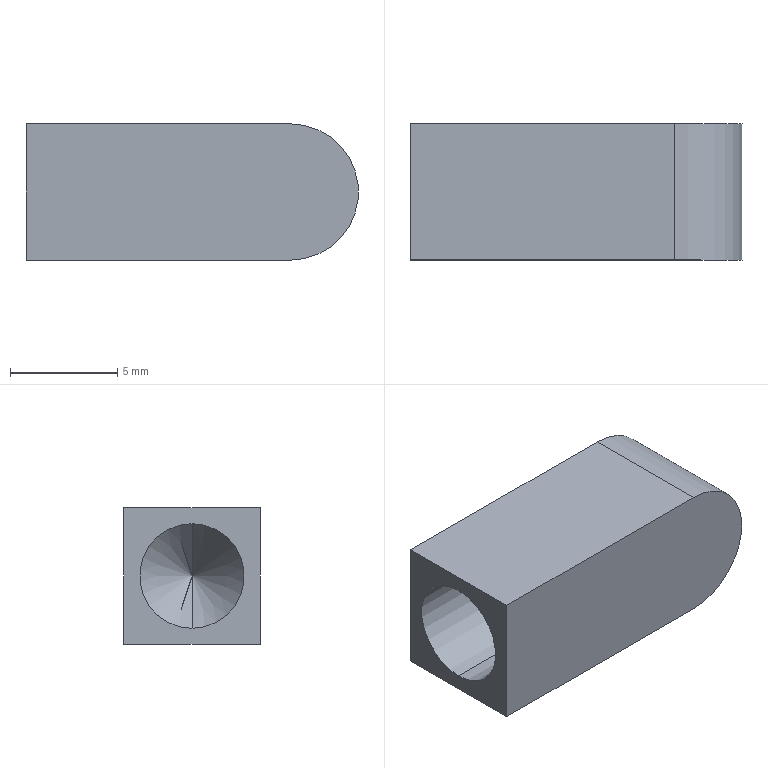Part | SolidWorks | features Extrusion 1, ICE 1, RevCut 1 | 1 solid | 10 faces | box 15.494 x 6.35 x 6.35 mm | volume 372.244 mm3 | plane 5 | cylinder 3 | cone 2 | commonest cylinder face diameters 4.877 x2 6.35 x1
STEP:
#1=CARTESIAN_POINT('',(0.5479,0.,0.));
#2=VERTEX_POINT('',#1);
#3=CARTESIAN_POINT('',(0.4375,0.,0.096));
#4=VERTEX_POINT('',#3);
#5=CARTESIAN_POINT('',(0.4375,0.,0.096));
#6=DIRECTION('',(-0.7547,0.,0.6561));
#7=VECTOR('',#6,39.37);
#8=LINE('',#5,#7);
#9=EDGE_CURVE('',#2,#4,#8,.T.);
#10=ORIENTED_EDGE('',*,*,#9,.F.);
#11=CARTESIAN_POINT('',(0.4375,0.,-0.096));
#12=VERTEX_POINT('',#11);
#13=CARTESIAN_POINT('',(0.4375,0.,-0.096));
#14=DIRECTION('',(-0.7547,0.,-0.6561));
#15=VECTOR('',#14,39.37);
#16=LINE('',#13,#15);
#17=EDGE_CURVE('',#2,#12,#16,.T.);
#18=ORIENTED_EDGE('',*,*,#17,.T.);
#19=CARTESIAN_POINT('',(0.4375,0.,0.));
#20=DIRECTION('',(-1.,0.,0.));
#21=DIRECTION('',(0.,0.,1.));
#22=AXIS2_PLACEMENT_3D('',#19,#20,#21);
#23=CIRCLE('',#22,0.096);
#24=EDGE_CURVE('',#12,#4,#23,.T.);
#25=ORIENTED_EDGE('',*,*,#24,.T.);
#26=EDGE_LOOP('',(#10,#18,#25));
#27=FACE_OUTER_BOUND('',#26,.T.);
#28=CARTESIAN_POINT('',(0.4375,0.,0.));
#29=DIRECTION('',(-1.,0.,0.));
#30=DIRECTION('',(0.,0.,1.));
#31=AXIS2_PLACEMENT_3D('',#28,#29,#30);
#32=CONICAL_SURFACE('',#31,0.096,0.7156);
#33=ADVANCED_FACE('',(#27),#32,.F.);
#34=ORIENTED_EDGE('',*,*,#24,.F.);
#35=CARTESIAN_POINT('',(0.,0.,-0.096));
#36=VERTEX_POINT('',#35);
#37=CARTESIAN_POINT('',(0.4375,0.,-0.096));
#38=DIRECTION('',(-1.,0.,0.));
#39=VECTOR('',#38,39.37);
#40=LINE('',#37,#39);
#41=EDGE_CURVE('',#12,#36,#40,.T.);
#42=ORIENTED_EDGE('',*,*,#41,.T.);
#43=CARTESIAN_POINT('',(0.,0.,0.096));
#44=VERTEX_POINT('',#43);
#45=CARTESIAN_POINT('',(0.,0.,0.));
#46=DIRECTION('',(-1.,0.,0.));
#47=DIRECTION('',(0.,0.,1.));
#48=AXIS2_PLACEMENT_3D('',#45,#46,#47);
#49=CIRCLE('',#48,0.096);
#50=EDGE_CURVE('',#36,#44,#49,.T.);
#51=ORIENTED_EDGE('',*,*,#50,.T.);
#52=CARTESIAN_POINT('',(0.4375,0.,0.096));
#53=DIRECTION('',(-1.,0.,0.));
#54=VECTOR('',#53,39.37);
#55=LINE('',#52,#54);
#56=EDGE_CURVE('',#4,#44,#55,.T.);
#57=ORIENTED_EDGE('',*,*,#56,.F.);
#58=EDGE_LOOP('',(#34,#42,#51,#57));
#59=FACE_OUTER_BOUND('',#58,.T.);
#60=CARTESIAN_POINT('',(0.4375,0.,0.));
#61=DIRECTION('',(-1.,0.,0.));
#62=DIRECTION('',(0.,0.,1.));
#63=AXIS2_PLACEMENT_3D('',#60,#61,#62);
#64=CYLINDRICAL_SURFACE('',#63,0.096);
#65=ADVANCED_FACE('',(#59),#64,.F.);
#66=CARTESIAN_POINT('',(0.,0.,0.));
#67=DIRECTION('',(-1.,0.,0.));
#68=DIRECTION('',(0.,0.,1.));
#69=AXIS2_PLACEMENT_3D('',#66,#67,#68);
#70=CIRCLE('',#69,0.096);
#71=EDGE_CURVE('',#44,#36,#70,.T.);
#72=ORIENTED_EDGE('',*,*,#71,.F.);
#73=ORIENTED_EDGE('',*,*,#50,.F.);
#74=EDGE_LOOP('',(#72,#73));
#75=FACE_BOUND('',#74,.T.);
#76=CARTESIAN_POINT('',(0.,-0.125,-0.125));
#77=VERTEX_POINT('',#76);
#78=CARTESIAN_POINT('',(0.,-0.125,0.125));
#79=VERTEX_POINT('',#78);
#80=CARTESIAN_POINT('',(0.,-0.125,-0.125));
#81=DIRECTION('',(0.,0.,1.));
#82=VECTOR('',#81,39.37);
#83=LINE('',#80,#82);
#84=EDGE_CURVE('',#77,#79,#83,.T.);
#85=ORIENTED_EDGE('',*,*,#84,.T.);
#86=CARTESIAN_POINT('',(0.,0.125,0.125));
#87=VERTEX_POINT('',#86);
#88=CARTESIAN_POINT('',(0.,0.125,0.125));
#89=DIRECTION('',(0.,-1.,0.));
#90=VECTOR('',#89,39.37);
#91=LINE('',#88,#90);
#92=EDGE_CURVE('',#87,#79,#91,.T.);
#93=ORIENTED_EDGE('',*,*,#92,.F.);
#94=CARTESIAN_POINT('',(0.,0.125,-0.125));
#95=VERTEX_POINT('',#94);
#96=CARTESIAN_POINT('',(0.,0.125,-0.125));
#97=DIRECTION('',(0.,0.,1.));
#98=VECTOR('',#97,39.37);
#99=LINE('',#96,#98);
#100=EDGE_CURVE('',#95,#87,#99,.T.);
#101=ORIENTED_EDGE('',*,*,#100,.F.);
#102=CARTESIAN_POINT('',(0.,0.125,-0.125));
#103=DIRECTION('',(0.,-1.,0.));
#104=VECTOR('',#103,39.37);
#105=LINE('',#102,#104);
#106=EDGE_CURVE('',#95,#77,#105,.T.);
#107=ORIENTED_EDGE('',*,*,#106,.T.);
#108=EDGE_LOOP('',(#85,#93,#101,#107));
#109=FACE_OUTER_BOUND('',#108,.T.);
#110=CARTESIAN_POINT('',(0.,0.125,-0.125));
#111=DIRECTION('',(1.,0.,0.));
#112=DIRECTION('',(0.,0.,-1.));
#113=AXIS2_PLACEMENT_3D('',#110,#111,#112);
#114=PLANE('',#113);
#115=ADVANCED_FACE('',(#75,#109),#114,.F.);
#116=CARTESIAN_POINT('',(0.485,-0.125,0.125));
#117=VERTEX_POINT('',#116);
#118=CARTESIAN_POINT('',(0.,-0.125,0.125));
#119=DIRECTION('',(1.,0.,0.));
#120=VECTOR('',#119,39.37);
#121=LINE('',#118,#120);
#122=EDGE_CURVE('',#79,#117,#121,.T.);
#123=ORIENTED_EDGE('',*,*,#122,.T.);
#124=CARTESIAN_POINT('',(0.485,0.125,0.125));
#125=VERTEX_POINT('',#124);
#126=CARTESIAN_POINT('',(0.485,0.125,0.125));
#127=DIRECTION('',(0.,-1.,0.));
#128=VECTOR('',#127,39.37);
#129=LINE('',#126,#128);
#130=EDGE_CURVE('',#125,#117,#129,.T.);
#131=ORIENTED_EDGE('',*,*,#130,.F.);
#132=CARTESIAN_POINT('',(0.,0.125,0.125));
#133=DIRECTION('',(1.,0.,0.));
#134=VECTOR('',#133,39.37);
#135=LINE('',#132,#134);
#136=EDGE_CURVE('',#87,#125,#135,.T.);
#137=ORIENTED_EDGE('',*,*,#136,.F.);
#138=ORIENTED_EDGE('',*,*,#92,.T.);
#139=EDGE_LOOP('',(#123,#131,#137,#138));
#140=FACE_OUTER_BOUND('',#139,.T.);
#141=CARTESIAN_POINT('',(0.,0.125,0.125));
#142=DIRECTION('',(0.,0.,-1.));
#143=DIRECTION('',(-1.,0.,0.));
#144=AXIS2_PLACEMENT_3D('',#141,#142,#143);
#145=PLANE('',#144);
#146=ADVANCED_FACE('',(#140),#145,.F.);
#147=CARTESIAN_POINT('',(0.485,-0.125,-0.125));
#148=VERTEX_POINT('',#147);
#149=CARTESIAN_POINT('',(0.485,-0.125,0.));
#150=DIRECTION('',(0.,1.,0.));
#151=DIRECTION('',(0.,0.,1.));
#152=AXIS2_PLACEMENT_3D('',#149,#150,#151);
#153=CIRCLE('',#152,0.125);
#154=EDGE_CURVE('',#117,#148,#153,.T.);
#155=ORIENTED_EDGE('',*,*,#154,.T.);
#156=CARTESIAN_POINT('',(0.485,0.125,-0.125));
#157=VERTEX_POINT('',#156);
#158=CARTESIAN_POINT('',(0.485,0.125,-0.125));
#159=DIRECTION('',(0.,-1.,0.));
#160=VECTOR('',#159,39.37);
#161=LINE('',#158,#160);
#162=EDGE_CURVE('',#157,#148,#161,.T.);
#163=ORIENTED_EDGE('',*,*,#162,.F.);
#164=CARTESIAN_POINT('',(0.485,0.125,0.));
#165=DIRECTION('',(0.,1.,0.));
#166=DIRECTION('',(0.,0.,1.));
#167=AXIS2_PLACEMENT_3D('',#164,#165,#166);
#168=CIRCLE('',#167,0.125);
#169=EDGE_CURVE('',#125,#157,#168,.T.);
#170=ORIENTED_EDGE('',*,*,#169,.F.);
#171=ORIENTED_EDGE('',*,*,#130,.T.);
#172=EDGE_LOOP('',(#155,#163,#170,#171));
#173=FACE_OUTER_BOUND('',#172,.T.);
#174=CARTESIAN_POINT('',(0.485,0.125,0.));
#175=DIRECTION('',(0.,-1.,0.));
#176=DIRECTION('',(0.,0.,-1.));
#177=AXIS2_PLACEMENT_3D('',#174,#175,#176);
#178=CYLINDRICAL_SURFACE('',#177,0.125);
#179=ADVANCED_FACE('',(#173),#178,.T.);
#180=CARTESIAN_POINT('',(0.,-0.125,-0.125));
#181=DIRECTION('',(-1.,0.,0.));
#182=VECTOR('',#181,39.37);
#183=LINE('',#180,#182);
#184=EDGE_CURVE('',#148,#77,#183,.T.);
#185=ORIENTED_EDGE('',*,*,#184,.T.);
#186=ORIENTED_EDGE('',*,*,#106,.F.);
#187=CARTESIAN_POINT('',(0.,0.125,-0.125));
#188=DIRECTION('',(-1.,0.,0.));
#189=VECTOR('',#188,39.37);
#190=LINE('',#187,#189);
#191=EDGE_CURVE('',#157,#95,#190,.T.);
#192=ORIENTED_EDGE('',*,*,#191,.F.);
#193=ORIENTED_EDGE('',*,*,#162,.T.);
#194=EDGE_LOOP('',(#185,#186,#192,#193));
#195=FACE_OUTER_BOUND('',#194,.T.);
#196=CARTESIAN_POINT('',(0.,0.125,-0.125));
#197=DIRECTION('',(0.,0.,1.));
#198=DIRECTION('',(1.,0.,0.));
#199=AXIS2_PLACEMENT_3D('',#196,#197,#198);
#200=PLANE('',#199);
#201=ADVANCED_FACE('',(#195),#200,.F.);
#202=ORIENTED_EDGE('',*,*,#100,.T.);
#203=ORIENTED_EDGE('',*,*,#136,.T.);
#204=ORIENTED_EDGE('',*,*,#169,.T.);
#205=ORIENTED_EDGE('',*,*,#191,.T.);
#206=EDGE_LOOP('',(#202,#203,#204,#205));
#207=FACE_OUTER_BOUND('',#206,.T.);
#208=CARTESIAN_POINT('',(0.485,0.125,0.));
#209=DIRECTION('',(0.,1.,0.));
#210=DIRECTION('',(0.,0.,1.));
#211=AXIS2_PLACEMENT_3D('',#208,#209,#210);
#212=PLANE('',#211);
#213=ADVANCED_FACE('',(#207),#212,.T.);
#214=ORIENTED_EDGE('',*,*,#84,.F.);
#215=ORIENTED_EDGE('',*,*,#184,.F.);
#216=ORIENTED_EDGE('',*,*,#154,.F.);
#217=ORIENTED_EDGE('',*,*,#122,.F.);
#218=EDGE_LOOP('',(#214,#215,#216,#217));
#219=FACE_OUTER_BOUND('',#218,.T.);
#220=CARTESIAN_POINT('',(0.485,-0.125,0.));
#221=DIRECTION('',(0.,1.,0.));
#222=DIRECTION('',(0.,0.,1.));
#223=AXIS2_PLACEMENT_3D('',#220,#221,#222);
#224=PLANE('',#223);
#225=ADVANCED_FACE('',(#219),#224,.F.);
#226=ORIENTED_EDGE('',*,*,#41,.F.);
#227=CARTESIAN_POINT('',(0.4375,0.,0.));
#228=DIRECTION('',(-1.,0.,0.));
#229=DIRECTION('',(0.,0.,1.));
#230=AXIS2_PLACEMENT_3D('',#227,#228,#229);
#231=CIRCLE('',#230,0.096);
#232=EDGE_CURVE('',#4,#12,#231,.T.);
#233=ORIENTED_EDGE('',*,*,#232,.F.);
#234=ORIENTED_EDGE('',*,*,#56,.T.);
#235=ORIENTED_EDGE('',*,*,#71,.T.);
#236=EDGE_LOOP('',(#226,#233,#234,#235));
#237=FACE_OUTER_BOUND('',#236,.T.);
#238=CARTESIAN_POINT('',(0.4375,0.,0.));
#239=DIRECTION('',(-1.,0.,0.));
#240=DIRECTION('',(0.,0.,1.));
#241=AXIS2_PLACEMENT_3D('',#238,#239,#240);
#242=CYLINDRICAL_SURFACE('',#241,0.096);
#243=ADVANCED_FACE('',(#237),#242,.F.);
#244=ORIENTED_EDGE('',*,*,#17,.F.);
#245=ORIENTED_EDGE('',*,*,#9,.T.);
#246=ORIENTED_EDGE('',*,*,#232,.T.);
#247=EDGE_LOOP('',(#244,#245,#246));
#248=FACE_OUTER_BOUND('',#247,.T.);
#249=CARTESIAN_POINT('',(0.4375,0.,0.));
#250=DIRECTION('',(-1.,0.,0.));
#251=DIRECTION('',(0.,0.,1.));
#252=AXIS2_PLACEMENT_3D('',#249,#250,#251);
#253=CONICAL_SURFACE('',#252,0.096,0.7156);
#254=ADVANCED_FACE('',(#248),#253,.F.);
#255=CLOSED_SHELL('',(#33,#65,#115,#146,#179,#201,#213,#225,#243,#254));
#256=MANIFOLD_SOLID_BREP('',#255);
#257=CARTESIAN_POINT('',(0.,0.,0.));
#258=DIRECTION('',(0.,0.,1.));
#259=DIRECTION('',(1.,0.,0.));
#260=AXIS2_PLACEMENT_3D('',#257,#258,#259);
#261=(LENGTH_UNIT()NAMED_UNIT(*)SI_UNIT($,.METRE.));
#262=LENGTH_MEASURE_WITH_UNIT(LENGTH_MEASURE(0.0254),#261);
#263=DIMENSIONAL_EXPONENTS(1.,0.,0.,0.,0.,0.,0.);
#264=(CONVERSION_BASED_UNIT('INCH',#262)LENGTH_UNIT()NAMED_UNIT(#263));
#265=UNCERTAINTY_MEASURE_WITH_UNIT(LENGTH_MEASURE(0.00001),#264,'','');
#266=(NAMED_UNIT(*)PLANE_ANGLE_UNIT()SI_UNIT($,.RADIAN.));
#267=(NAMED_UNIT(*)SI_UNIT($,.STERADIAN.)SOLID_ANGLE_UNIT());
#268=(GEOMETRIC_REPRESENTATION_CONTEXT(3)GLOBAL_UNCERTAINTY_ASSIGNED_CONTEXT((#265))GLOBAL_UNIT_ASSIGNED_CONTEXT((#264,#266,#267))REPRESENTATION_CONTEXT('',''));
#269=ADVANCED_BREP_SHAPE_REPRESENTATION('',(#256,#260),#268);